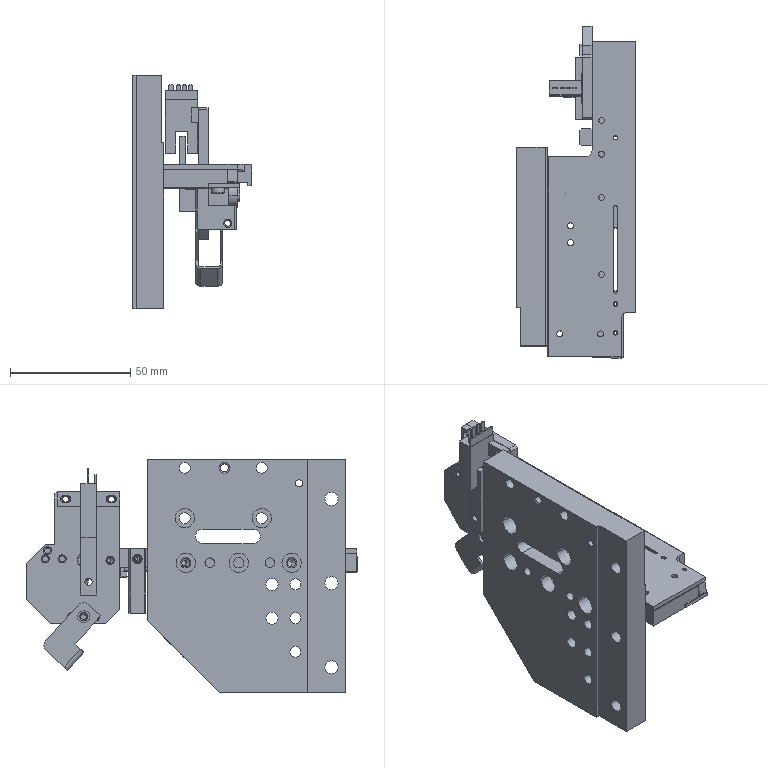Part | NX | 19 solids | 1269 faces | box 49.55 x 138 x 97 mm | volume 132374 mm3 | plane 890 | cylinder 247 | cone 124 | torus 8 | commonest cylinder face diameters 2.5 x60 3 x22 4 x18 5.5 x18 1.5 x15 4.6 x14